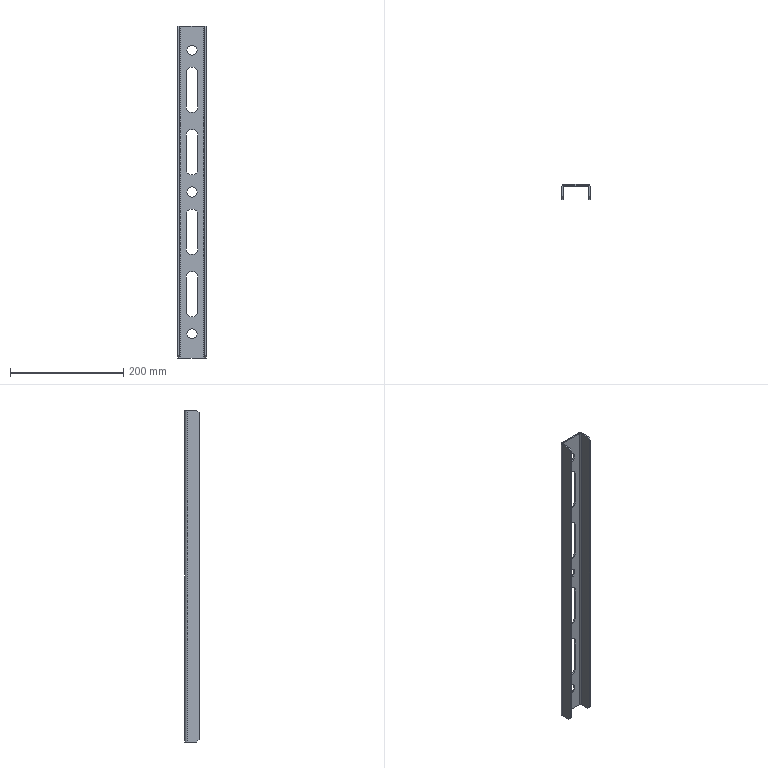Part | SolidWorks | features Chamfer 1, FlatPattern 1, ICE 1, SMBaseFlange 1, SheetMetal 1 | 1 solid | 48 faces | box 50 x 26 x 585.4 mm | volume 111122 mm3 | plane 30 | cylinder 18 | commonest cylinder face diameters 20 x8 18 x6 5 x2 9.6 x2
STEP:
#1=CARTESIAN_POINT('',(-9.,-2.3,-250.));
#2=VERTEX_POINT('',#1);
#3=CARTESIAN_POINT('',(9.,-2.3,-250.));
#4=VERTEX_POINT('',#3);
#5=CARTESIAN_POINT('',(0.,-2.3,-250.));
#6=DIRECTION('',(0.,-1.,0.));
#7=DIRECTION('',(1.,0.,0.));
#8=AXIS2_PLACEMENT_3D('',#5,#6,#7);
#9=CIRCLE('',#8,9.);
#10=EDGE_CURVE('',#2,#4,#9,.T.);
#11=ORIENTED_EDGE('',*,*,#10,.T.);
#12=CARTESIAN_POINT('',(9.,0.,-250.));
#13=VERTEX_POINT('',#12);
#14=CARTESIAN_POINT('',(9.,-26.,-250.));
#15=DIRECTION('',(0.,1.,0.));
#16=VECTOR('',#15,1000.);
#17=LINE('',#14,#16);
#18=EDGE_CURVE('',#4,#13,#17,.T.);
#19=ORIENTED_EDGE('',*,*,#18,.T.);
#20=CARTESIAN_POINT('',(-9.,0.,-250.));
#21=VERTEX_POINT('',#20);
#22=CARTESIAN_POINT('',(0.,0.,-250.));
#23=DIRECTION('',(0.,1.,0.));
#24=DIRECTION('',(1.,0.,0.));
#25=AXIS2_PLACEMENT_3D('',#22,#23,#24);
#26=CIRCLE('',#25,9.);
#27=EDGE_CURVE('',#13,#21,#26,.T.);
#28=ORIENTED_EDGE('',*,*,#27,.T.);
#29=CARTESIAN_POINT('',(-9.,-26.,-250.));
#30=DIRECTION('',(0.,1.,0.));
#31=VECTOR('',#30,1000.);
#32=LINE('',#29,#31);
#33=EDGE_CURVE('',#2,#21,#32,.T.);
#34=ORIENTED_EDGE('',*,*,#33,.F.);
#35=EDGE_LOOP('',(#11,#19,#28,#34));
#36=FACE_OUTER_BOUND('',#35,.T.);
#37=CARTESIAN_POINT('',(0.,-26.,-250.));
#38=DIRECTION('',(0.,1.,0.));
#39=DIRECTION('',(-1.,0.,0.));
#40=AXIS2_PLACEMENT_3D('',#37,#38,#39);
#41=CYLINDRICAL_SURFACE('',#40,9.);
#42=ADVANCED_FACE('',(#36),#41,.F.);
#43=CARTESIAN_POINT('',(-9.,-2.3,250.));
#44=VERTEX_POINT('',#43);
#45=CARTESIAN_POINT('',(9.,-2.3,250.));
#46=VERTEX_POINT('',#45);
#47=CARTESIAN_POINT('',(0.,-2.3,250.));
#48=DIRECTION('',(0.,-1.,0.));
#49=DIRECTION('',(1.,0.,0.));
#50=AXIS2_PLACEMENT_3D('',#47,#48,#49);
#51=CIRCLE('',#50,9.);
#52=EDGE_CURVE('',#44,#46,#51,.T.);
#53=ORIENTED_EDGE('',*,*,#52,.T.);
#54=CARTESIAN_POINT('',(9.,0.,250.));
#55=VERTEX_POINT('',#54);
#56=CARTESIAN_POINT('',(9.,-26.,250.));
#57=DIRECTION('',(0.,1.,0.));
#58=VECTOR('',#57,1000.);
#59=LINE('',#56,#58);
#60=EDGE_CURVE('',#46,#55,#59,.T.);
#61=ORIENTED_EDGE('',*,*,#60,.T.);
#62=CARTESIAN_POINT('',(-9.,0.,250.));
#63=VERTEX_POINT('',#62);
#64=CARTESIAN_POINT('',(0.,0.,250.));
#65=DIRECTION('',(0.,1.,0.));
#66=DIRECTION('',(-1.,0.,0.));
#67=AXIS2_PLACEMENT_3D('',#64,#65,#66);
#68=CIRCLE('',#67,9.);
#69=EDGE_CURVE('',#55,#63,#68,.T.);
#70=ORIENTED_EDGE('',*,*,#69,.T.);
#71=CARTESIAN_POINT('',(-9.,-26.,250.));
#72=DIRECTION('',(0.,1.,0.));
#73=VECTOR('',#72,1000.);
#74=LINE('',#71,#73);
#75=EDGE_CURVE('',#44,#63,#74,.T.);
#76=ORIENTED_EDGE('',*,*,#75,.F.);
#77=EDGE_LOOP('',(#53,#61,#70,#76));
#78=FACE_OUTER_BOUND('',#77,.T.);
#79=CARTESIAN_POINT('',(0.,-26.,250.));
#80=DIRECTION('',(0.,1.,0.));
#81=DIRECTION('',(-1.,0.,0.));
#82=AXIS2_PLACEMENT_3D('',#79,#80,#81);
#83=CYLINDRICAL_SURFACE('',#82,9.);
#84=ADVANCED_FACE('',(#78),#83,.F.);
#85=CARTESIAN_POINT('',(-9.,-2.3,0.));
#86=VERTEX_POINT('',#85);
#87=CARTESIAN_POINT('',(9.,-2.3,0.));
#88=VERTEX_POINT('',#87);
#89=CARTESIAN_POINT('',(0.,-2.3,0.));
#90=DIRECTION('',(0.,-1.,0.));
#91=DIRECTION('',(1.,0.,0.));
#92=AXIS2_PLACEMENT_3D('',#89,#90,#91);
#93=CIRCLE('',#92,9.);
#94=EDGE_CURVE('',#86,#88,#93,.T.);
#95=ORIENTED_EDGE('',*,*,#94,.T.);
#96=CARTESIAN_POINT('',(9.,0.,0.));
#97=VERTEX_POINT('',#96);
#98=CARTESIAN_POINT('',(9.,-26.,0.));
#99=DIRECTION('',(0.,1.,0.));
#100=VECTOR('',#99,1000.);
#101=LINE('',#98,#100);
#102=EDGE_CURVE('',#88,#97,#101,.T.);
#103=ORIENTED_EDGE('',*,*,#102,.T.);
#104=CARTESIAN_POINT('',(-9.,0.,0.));
#105=VERTEX_POINT('',#104);
#106=CARTESIAN_POINT('',(0.,0.,0.));
#107=DIRECTION('',(0.,1.,0.));
#108=DIRECTION('',(-1.,0.,0.));
#109=AXIS2_PLACEMENT_3D('',#106,#107,#108);
#110=CIRCLE('',#109,9.);
#111=EDGE_CURVE('',#97,#105,#110,.T.);
#112=ORIENTED_EDGE('',*,*,#111,.T.);
#113=CARTESIAN_POINT('',(-9.,-26.,0.));
#114=DIRECTION('',(0.,1.,0.));
#115=VECTOR('',#114,1000.);
#116=LINE('',#113,#115);
#117=EDGE_CURVE('',#86,#105,#116,.T.);
#118=ORIENTED_EDGE('',*,*,#117,.F.);
#119=EDGE_LOOP('',(#95,#103,#112,#118));
#120=FACE_OUTER_BOUND('',#119,.T.);
#121=CARTESIAN_POINT('',(0.,-26.,0.));
#122=DIRECTION('',(0.,1.,0.));
#123=DIRECTION('',(-1.,0.,0.));
#124=AXIS2_PLACEMENT_3D('',#121,#122,#123);
#125=CYLINDRICAL_SURFACE('',#124,9.);
#126=ADVANCED_FACE('',(#120),#125,.F.);
#127=CARTESIAN_POINT('',(25.,-4.8,292.7));
#128=VERTEX_POINT('',#127);
#129=CARTESIAN_POINT('',(22.7,-4.8,292.7));
#130=VERTEX_POINT('',#129);
#131=CARTESIAN_POINT('',(25.,-4.8,292.7));
#132=DIRECTION('',(-1.,0.,0.));
#133=VECTOR('',#132,1000.);
#134=LINE('',#131,#133);
#135=EDGE_CURVE('',#128,#130,#134,.T.);
#136=ORIENTED_EDGE('',*,*,#135,.F.);
#137=CARTESIAN_POINT('',(20.2,0.,292.7));
#138=VERTEX_POINT('',#137);
#139=CARTESIAN_POINT('',(20.2,-4.8,292.7));
#140=DIRECTION('',(0.,0.,1.));
#141=DIRECTION('',(-1.,0.,0.));
#142=AXIS2_PLACEMENT_3D('',#139,#140,#141);
#143=CIRCLE('',#142,4.8);
#144=EDGE_CURVE('',#128,#138,#143,.T.);
#145=ORIENTED_EDGE('',*,*,#144,.T.);
#146=CARTESIAN_POINT('',(20.2,-2.3,292.7));
#147=VERTEX_POINT('',#146);
#148=CARTESIAN_POINT('',(20.2,-2.3,292.7));
#149=DIRECTION('',(0.,1.,0.));
#150=VECTOR('',#149,1000.);
#151=LINE('',#148,#150);
#152=EDGE_CURVE('',#147,#138,#151,.T.);
#153=ORIENTED_EDGE('',*,*,#152,.F.);
#154=CARTESIAN_POINT('',(20.2,-4.8,292.7));
#155=DIRECTION('',(0.,0.,1.));
#156=DIRECTION('',(1.,0.,0.));
#157=AXIS2_PLACEMENT_3D('',#154,#155,#156);
#158=CIRCLE('',#157,2.5);
#159=EDGE_CURVE('',#130,#147,#158,.T.);
#160=ORIENTED_EDGE('',*,*,#159,.F.);
#161=EDGE_LOOP('',(#136,#145,#153,#160));
#162=FACE_OUTER_BOUND('',#161,.T.);
#163=CARTESIAN_POINT('',(25.,-4.8,292.7));
#164=DIRECTION('',(0.,0.,1.));
#165=DIRECTION('',(1.,0.,0.));
#166=AXIS2_PLACEMENT_3D('',#163,#164,#165);
#167=PLANE('',#166);
#168=ADVANCED_FACE('',(#162),#167,.T.);
#169=CARTESIAN_POINT('',(22.7,-21.,292.7));
#170=VERTEX_POINT('',#169);
#171=CARTESIAN_POINT('',(22.7,0.,292.7));
#172=DIRECTION('',(0.,1.,0.));
#173=VECTOR('',#172,1000.);
#174=LINE('',#171,#173);
#175=EDGE_CURVE('',#170,#130,#174,.T.);
#176=ORIENTED_EDGE('',*,*,#175,.F.);
#177=CARTESIAN_POINT('',(25.,-21.,292.7));
#178=VERTEX_POINT('',#177);
#179=CARTESIAN_POINT('',(20.2,-21.,292.7));
#180=DIRECTION('',(1.,0.,0.));
#181=VECTOR('',#180,1000.);
#182=LINE('',#179,#181);
#183=EDGE_CURVE('',#170,#178,#182,.T.);
#184=ORIENTED_EDGE('',*,*,#183,.T.);
#185=CARTESIAN_POINT('',(25.,0.,292.7));
#186=DIRECTION('',(0.,1.,0.));
#187=VECTOR('',#186,1000.);
#188=LINE('',#185,#187);
#189=EDGE_CURVE('',#178,#128,#188,.T.);
#190=ORIENTED_EDGE('',*,*,#189,.T.);
#191=ORIENTED_EDGE('',*,*,#135,.T.);
#192=EDGE_LOOP('',(#176,#184,#190,#191));
#193=FACE_OUTER_BOUND('',#192,.T.);
#194=CARTESIAN_POINT('',(20.2,-2.3,292.7));
#195=DIRECTION('',(0.,0.,1.));
#196=DIRECTION('',(1.,0.,0.));
#197=AXIS2_PLACEMENT_3D('',#194,#195,#196);
#198=PLANE('',#197);
#199=ADVANCED_FACE('',(#193),#198,.T.);
#200=CARTESIAN_POINT('',(20.2,0.,-292.7));
#201=VERTEX_POINT('',#200);
#202=CARTESIAN_POINT('',(20.2,-2.3,-292.7));
#203=VERTEX_POINT('',#202);
#204=CARTESIAN_POINT('',(20.2,0.,-292.7));
#205=DIRECTION('',(0.,-1.,0.));
#206=VECTOR('',#205,1000.);
#207=LINE('',#204,#206);
#208=EDGE_CURVE('',#201,#203,#207,.T.);
#209=ORIENTED_EDGE('',*,*,#208,.F.);
#210=CARTESIAN_POINT('',(25.,-4.8,-292.7));
#211=VERTEX_POINT('',#210);
#212=CARTESIAN_POINT('',(20.2,-4.8,-292.7));
#213=DIRECTION('',(0.,0.,1.));
#214=DIRECTION('',(-1.,0.,0.));
#215=AXIS2_PLACEMENT_3D('',#212,#213,#214);
#216=CIRCLE('',#215,4.8);
#217=EDGE_CURVE('',#211,#201,#216,.T.);
#218=ORIENTED_EDGE('',*,*,#217,.F.);
#219=CARTESIAN_POINT('',(22.7,-4.8,-292.7));
#220=VERTEX_POINT('',#219);
#221=CARTESIAN_POINT('',(22.7,-4.8,-292.7));
#222=DIRECTION('',(1.,0.,0.));
#223=VECTOR('',#222,1000.);
#224=LINE('',#221,#223);
#225=EDGE_CURVE('',#220,#211,#224,.T.);
#226=ORIENTED_EDGE('',*,*,#225,.F.);
#227=CARTESIAN_POINT('',(20.2,-4.8,-292.7));
#228=DIRECTION('',(0.,0.,1.));
#229=DIRECTION('',(1.,0.,0.));
#230=AXIS2_PLACEMENT_3D('',#227,#228,#229);
#231=CIRCLE('',#230,2.5);
#232=EDGE_CURVE('',#220,#203,#231,.T.);
#233=ORIENTED_EDGE('',*,*,#232,.T.);
#234=EDGE_LOOP('',(#209,#218,#226,#233));
#235=FACE_OUTER_BOUND('',#234,.T.);
#236=CARTESIAN_POINT('',(20.2,0.,-292.7));
#237=DIRECTION('',(0.,0.,-1.));
#238=DIRECTION('',(-1.,0.,0.));
#239=AXIS2_PLACEMENT_3D('',#236,#237,#238);
#240=PLANE('',#239);
#241=ADVANCED_FACE('',(#235),#240,.T.);
#242=CARTESIAN_POINT('',(-20.2,0.,-292.7));
#243=VERTEX_POINT('',#242);
#244=CARTESIAN_POINT('',(-25.,0.,-292.7));
#245=DIRECTION('',(-1.,0.,0.));
#246=VECTOR('',#245,1000.);
#247=LINE('',#244,#246);
#248=EDGE_CURVE('',#201,#243,#247,.T.);
#249=ORIENTED_EDGE('',*,*,#248,.F.);
#250=ORIENTED_EDGE('',*,*,#208,.T.);
#251=CARTESIAN_POINT('',(-20.2,-2.3,-292.7));
#252=VERTEX_POINT('',#251);
#253=CARTESIAN_POINT('',(-25.,-2.3,-292.7));
#254=DIRECTION('',(-1.,0.,0.));
#255=VECTOR('',#254,1000.);
#256=LINE('',#253,#255);
#257=EDGE_CURVE('',#203,#252,#256,.T.);
#258=ORIENTED_EDGE('',*,*,#257,.T.);
#259=CARTESIAN_POINT('',(-20.2,-2.3,-292.7));
#260=DIRECTION('',(0.,1.,0.));
#261=VECTOR('',#260,1000.);
#262=LINE('',#259,#261);
#263=EDGE_CURVE('',#252,#243,#262,.T.);
#264=ORIENTED_EDGE('',*,*,#263,.T.);
#265=EDGE_LOOP('',(#249,#250,#258,#264));
#266=FACE_OUTER_BOUND('',#265,.T.);
#267=CARTESIAN_POINT('',(22.7,-4.8,-292.7));
#268=DIRECTION('',(0.,0.,-1.));
#269=DIRECTION('',(-1.,0.,0.));
#270=AXIS2_PLACEMENT_3D('',#267,#268,#269);
#271=PLANE('',#270);
#272=ADVANCED_FACE('',(#266),#271,.T.);
#273=CARTESIAN_POINT('',(-20.2,0.,292.7));
#274=VERTEX_POINT('',#273);
#275=CARTESIAN_POINT('',(-20.2,-2.3,292.7));
#276=VERTEX_POINT('',#275);
#277=CARTESIAN_POINT('',(-20.2,0.,292.7));
#278=DIRECTION('',(0.,-1.,0.));
#279=VECTOR('',#278,1000.);
#280=LINE('',#277,#279);
#281=EDGE_CURVE('',#274,#276,#280,.T.);
#282=ORIENTED_EDGE('',*,*,#281,.F.);
#283=CARTESIAN_POINT('',(-25.,-4.8,292.7));
#284=VERTEX_POINT('',#283);
#285=CARTESIAN_POINT('',(-20.2,-4.8,292.7));
#286=DIRECTION('',(0.,0.,1.));
#287=DIRECTION('',(-1.,0.,0.));
#288=AXIS2_PLACEMENT_3D('',#285,#286,#287);
#289=CIRCLE('',#288,4.8);
#290=EDGE_CURVE('',#274,#284,#289,.T.);
#291=ORIENTED_EDGE('',*,*,#290,.T.);
#292=CARTESIAN_POINT('',(-22.7,-4.8,292.7));
#293=VERTEX_POINT('',#292);
#294=CARTESIAN_POINT('',(-22.7,-4.8,292.7));
#295=DIRECTION('',(-1.,0.,0.));
#296=VECTOR('',#295,1000.);
#297=LINE('',#294,#296);
#298=EDGE_CURVE('',#293,#284,#297,.T.);
#299=ORIENTED_EDGE('',*,*,#298,.F.);
#300=CARTESIAN_POINT('',(-20.2,-4.8,292.7));
#301=DIRECTION('',(0.,0.,1.));
#302=DIRECTION('',(1.,0.,0.));
#303=AXIS2_PLACEMENT_3D('',#300,#301,#302);
#304=CIRCLE('',#303,2.5);
#305=EDGE_CURVE('',#276,#293,#304,.T.);
#306=ORIENTED_EDGE('',*,*,#305,.F.);
#307=EDGE_LOOP('',(#282,#291,#299,#306));
#308=FACE_OUTER_BOUND('',#307,.T.);
#309=CARTESIAN_POINT('',(-20.2,0.,292.7));
#310=DIRECTION('',(0.,0.,1.));
#311=DIRECTION('',(1.,0.,0.));
#312=AXIS2_PLACEMENT_3D('',#309,#310,#311);
#313=PLANE('',#312);
#314=ADVANCED_FACE('',(#308),#313,.T.);
#315=CARTESIAN_POINT('',(-25.,0.,292.7));
#316=DIRECTION('',(-1.,0.,0.));
#317=VECTOR('',#316,1000.);
#318=LINE('',#315,#317);
#319=EDGE_CURVE('',#138,#274,#318,.T.);
#320=ORIENTED_EDGE('',*,*,#319,.T.);
#321=ORIENTED_EDGE('',*,*,#281,.T.);
#322=CARTESIAN_POINT('',(-25.,-2.3,292.7));
#323=DIRECTION('',(-1.,0.,0.));
#324=VECTOR('',#323,1000.);
#325=LINE('',#322,#324);
#326=EDGE_CURVE('',#147,#276,#325,.T.);
#327=ORIENTED_EDGE('',*,*,#326,.F.);
#328=ORIENTED_EDGE('',*,*,#152,.T.);
#329=EDGE_LOOP('',(#320,#321,#327,#328));
#330=FACE_OUTER_BOUND('',#329,.T.);
#331=CARTESIAN_POINT('',(-22.7,-4.8,292.7));
#332=DIRECTION('',(0.,0.,1.));
#333=DIRECTION('',(1.,0.,0.));
#334=AXIS2_PLACEMENT_3D('',#331,#332,#333);
#335=PLANE('',#334);
#336=ADVANCED_FACE('',(#330),#335,.T.);
#337=CARTESIAN_POINT('',(-25.,-4.8,-292.7));
#338=VERTEX_POINT('',#337);
#339=CARTESIAN_POINT('',(-22.7,-4.8,-292.7));
#340=VERTEX_POINT('',#339);
#341=CARTESIAN_POINT('',(-25.,-4.8,-292.7));
#342=DIRECTION('',(1.,0.,0.));
#343=VECTOR('',#342,1000.);
#344=LINE('',#341,#343);
#345=EDGE_CURVE('',#338,#340,#344,.T.);
#346=ORIENTED_EDGE('',*,*,#345,.F.);
#347=CARTESIAN_POINT('',(-20.2,-4.8,-292.7));
#348=DIRECTION('',(0.,0.,1.));
#349=DIRECTION('',(-1.,0.,0.));
#350=AXIS2_PLACEMENT_3D('',#347,#348,#349);
#351=CIRCLE('',#350,4.8);
#352=EDGE_CURVE('',#243,#338,#351,.T.);
#353=ORIENTED_EDGE('',*,*,#352,.F.);
#354=ORIENTED_EDGE('',*,*,#263,.F.);
#355=CARTESIAN_POINT('',(-20.2,-4.8,-292.7));
#356=DIRECTION('',(0.,0.,1.));
#357=DIRECTION('',(1.,0.,0.));
#358=AXIS2_PLACEMENT_3D('',#355,#356,#357);
#359=CIRCLE('',#358,2.5);
#360=EDGE_CURVE('',#252,#340,#359,.T.);
#361=ORIENTED_EDGE('',*,*,#360,.T.);
#362=EDGE_LOOP('',(#346,#353,#354,#361));
#363=FACE_OUTER_BOUND('',#362,.T.);
#364=CARTESIAN_POINT('',(-25.,-4.8,-292.7));
#365=DIRECTION('',(0.,0.,-1.));
#366=DIRECTION('',(-1.,0.,0.));
#367=AXIS2_PLACEMENT_3D('',#364,#365,#366);
#368=PLANE('',#367);
#369=ADVANCED_FACE('',(#363),#368,.T.);
#370=CARTESIAN_POINT('',(-22.7,-21.,-292.7));
#371=VERTEX_POINT('',#370);
#372=CARTESIAN_POINT('',(-22.7,0.,-292.7));
#373=DIRECTION('',(0.,-1.,0.));
#374=VECTOR('',#373,1000.);
#375=LINE('',#372,#374);
#376=EDGE_CURVE('',#340,#371,#375,.T.);
#377=ORIENTED_EDGE('',*,*,#376,.T.);
#378=CARTESIAN_POINT('',(-25.,-21.,-292.7));
#379=VERTEX_POINT('',#378);
#380=CARTESIAN_POINT('',(-20.2,-21.,-292.7));
#381=DIRECTION('',(-1.,0.,0.));
#382=VECTOR('',#381,1000.);
#383=LINE('',#380,#382);
#384=EDGE_CURVE('',#371,#379,#383,.T.);
#385=ORIENTED_EDGE('',*,*,#384,.T.);
#386=CARTESIAN_POINT('',(-25.,0.,-292.7));
#387=DIRECTION('',(0.,-1.,0.));
#388=VECTOR('',#387,1000.);
#389=LINE('',#386,#388);
#390=EDGE_CURVE('',#338,#379,#389,.T.);
#391=ORIENTED_EDGE('',*,*,#390,.F.);
#392=ORIENTED_EDGE('',*,*,#345,.T.);
#393=EDGE_LOOP('',(#377,#385,#391,#392));
#394=FACE_OUTER_BOUND('',#393,.T.);
#395=CARTESIAN_POINT('',(-20.2,-2.3,-292.7));
#396=DIRECTION('',(0.,0.,-1.));
#397=DIRECTION('',(-1.,0.,0.));
#398=AXIS2_PLACEMENT_3D('',#395,#396,#397);
#399=PLANE('',#398);
#400=ADVANCED_FACE('',(#394),#399,.T.);
#401=ORIENTED_EDGE('',*,*,#390,.T.);
#402=CARTESIAN_POINT('',(-25.,-26.,-287.7));
#403=VERTEX_POINT('',#402);
#404=CARTESIAN_POINT('',(-25.,-21.,-292.7));
#405=DIRECTION('',(0.,-0.7071,0.7071));
#406=VECTOR('',#405,1000.);
#407=LINE('',#404,#406);
#408=EDGE_CURVE('',#379,#403,#407,.T.);
#409=ORIENTED_EDGE('',*,*,#408,.T.);
#410=CARTESIAN_POINT('',(-25.,-26.,287.7));
#411=VERTEX_POINT('',#410);
#412=CARTESIAN_POINT('',(-25.,-26.,292.7));
#413=DIRECTION('',(0.,0.,-1.));
#414=VECTOR('',#413,1000.);
#415=LINE('',#412,#414);
#416=EDGE_CURVE('',#411,#403,#415,.T.);
#417=ORIENTED_EDGE('',*,*,#416,.F.);
#418=CARTESIAN_POINT('',(-25.,-21.,292.7));
#419=VERTEX_POINT('',#418);
#420=CARTESIAN_POINT('',(-25.,-26.,287.7));
#421=DIRECTION('',(0.,0.7071,0.7071));
#422=VECTOR('',#421,1000.);
#423=LINE('',#420,#422);
#424=EDGE_CURVE('',#411,#419,#423,.T.);
#425=ORIENTED_EDGE('',*,*,#424,.T.);
#426=CARTESIAN_POINT('',(-25.,0.,292.7));
#427=DIRECTION('',(0.,-1.,0.));
#428=VECTOR('',#427,1000.);
#429=LINE('',#426,#428);
#430=EDGE_CURVE('',#284,#419,#429,.T.);
#431=ORIENTED_EDGE('',*,*,#430,.F.);
#432=CARTESIAN_POINT('',(-25.,-4.8,292.7));
#433=DIRECTION('',(0.,0.,-1.));
#434=VECTOR('',#433,1000.);
#435=LINE('',#432,#434);
#436=EDGE_CURVE('',#284,#338,#435,.T.);
#437=ORIENTED_EDGE('',*,*,#436,.T.);
#438=EDGE_LOOP('',(#401,#409,#417,#425,#431,#437));
#439=FACE_OUTER_BOUND('',#438,.T.);
#440=CARTESIAN_POINT('',(-25.,0.,292.7));
#441=DIRECTION('',(1.,0.,0.));
#442=DIRECTION('',(0.,0.,-1.));
#443=AXIS2_PLACEMENT_3D('',#440,#441,#442);
#444=PLANE('',#443);
#445=ADVANCED_FACE('',(#439),#444,.F.);
#446=ORIENTED_EDGE('',*,*,#416,.T.);
#447=CARTESIAN_POINT('',(-22.7,-26.,-287.7));
#448=VERTEX_POINT('',#447);
#449=CARTESIAN_POINT('',(-22.7,-26.,-287.7));
#450=DIRECTION('',(1.,0.,0.));
#451=VECTOR('',#450,1000.);
#452=LINE('',#449,#451);
#453=EDGE_CURVE('',#403,#448,#452,.T.);
#454=ORIENTED_EDGE('',*,*,#453,.T.);
#455=CARTESIAN_POINT('',(-22.7,-26.,287.7));
#456=VERTEX_POINT('',#455);
#457=CARTESIAN_POINT('',(-22.7,-26.,292.7));
#458=DIRECTION('',(0.,0.,-1.));
#459=VECTOR('',#458,1000.);
#460=LINE('',#457,#459);
#461=EDGE_CURVE('',#456,#448,#460,.T.);
#462=ORIENTED_EDGE('',*,*,#461,.F.);
#463=CARTESIAN_POINT('',(-22.7,-26.,287.7));
#464=DIRECTION('',(-1.,0.,0.));
#465=VECTOR('',#464,1000.);
#466=LINE('',#463,#465);
#467=EDGE_CURVE('',#456,#411,#466,.T.);
#468=ORIENTED_EDGE('',*,*,#467,.T.);
#469=EDGE_LOOP('',(#446,#454,#462,#468));
#470=FACE_OUTER_BOUND('',#469,.T.);
#471=CARTESIAN_POINT('',(-22.7,-26.,292.7));
#472=DIRECTION('',(0.,-1.,0.));
#473=DIRECTION('',(0.,0.,-1.));
#474=AXIS2_PLACEMENT_3D('',#471,#472,#473);
#475=PLANE('',#474);
#476=ADVANCED_FACE('',(#470),#475,.T.);
#477=ORIENTED_EDGE('',*,*,#461,.T.);
#478=CARTESIAN_POINT('',(-22.7,-303.2,-10.5));
#479=DIRECTION('',(0.,0.7071,-0.7071));
#480=VECTOR('',#479,1000.);
#481=LINE('',#478,#480);
#482=EDGE_CURVE('',#448,#371,#481,.T.);
#483=ORIENTED_EDGE('',*,*,#482,.T.);
#484=ORIENTED_EDGE('',*,*,#376,.F.);
#485=CARTESIAN_POINT('',(-22.7,-4.8,292.7));
#486=DIRECTION('',(0.,0.,-1.));
#487=VECTOR('',#486,1000.);
#488=LINE('',#485,#487);
#489=EDGE_CURVE('',#293,#340,#488,.T.);
#490=ORIENTED_EDGE('',*,*,#489,.F.);
#491=CARTESIAN_POINT('',(-22.7,-21.,292.7));
#492=VERTEX_POINT('',#491);
#493=CARTESIAN_POINT('',(-22.7,0.,292.7));
#494=DIRECTION('',(0.,-1.,0.));
#495=VECTOR('',#494,1000.);
#496=LINE('',#493,#495);
#497=EDGE_CURVE('',#293,#492,#496,.T.);
#498=ORIENTED_EDGE('',*,*,#497,.T.);
#499=CARTESIAN_POINT('',(-22.7,-10.5,303.2));
#500=DIRECTION('',(0.,-0.7071,-0.7071));
#501=VECTOR('',#500,1000.);
#502=LINE('',#499,#501);
#503=EDGE_CURVE('',#492,#456,#502,.T.);
#504=ORIENTED_EDGE('',*,*,#503,.T.);
#505=EDGE_LOOP('',(#477,#483,#484,#490,#498,#504));
#506=FACE_OUTER_BOUND('',#505,.T.);
#507=CARTESIAN_POINT('',(-22.7,0.,292.7));
#508=DIRECTION('',(1.,0.,0.));
#509=DIRECTION('',(0.,0.,-1.));
#510=AXIS2_PLACEMENT_3D('',#507,#508,#509);
#511=PLANE('',#510);
#512=ADVANCED_FACE('',(#506),#511,.T.);
#513=ORIENTED_EDGE('',*,*,#360,.F.);
#514=CARTESIAN_POINT('',(-20.2,-2.3,292.7));
#515=DIRECTION('',(0.,0.,-1.));
#516=VECTOR('',#515,1000.);
#517=LINE('',#514,#516);
#518=EDGE_CURVE('',#276,#252,#517,.T.);
#519=ORIENTED_EDGE('',*,*,#518,.F.);
#520=ORIENTED_EDGE('',*,*,#305,.T.);
#521=ORIENTED_EDGE('',*,*,#489,.T.);
#522=EDGE_LOOP('',(#513,#519,#520,#521));
#523=FACE_OUTER_BOUND('',#522,.T.);
#524=CARTESIAN_POINT('',(-20.2,-4.8,292.7));
#525=DIRECTION('',(0.,0.,-1.));
#526=DIRECTION('',(-1.,0.,0.));
#527=AXIS2_PLACEMENT_3D('',#524,#525,#526);
#528=CYLINDRICAL_SURFACE('',#527,2.5);
#529=ADVANCED_FACE('',(#523),#528,.F.);
#530=ORIENTED_EDGE('',*,*,#10,.F.);
#531=CARTESIAN_POINT('',(0.,-2.3,-250.));
#532=DIRECTION('',(0.,-1.,0.));
#533=DIRECTION('',(1.,0.,0.));
#534=AXIS2_PLACEMENT_3D('',#531,#532,#533);
#535=CIRCLE('',#534,9.);
#536=EDGE_CURVE('',#4,#2,#535,.T.);
#537=ORIENTED_EDGE('',*,*,#536,.F.);
#538=EDGE_LOOP('',(#530,#537));
#539=FACE_BOUND('',#538,.T.);
#540=CARTESIAN_POINT('',(10.,-2.3,-150.));
#541=VERTEX_POINT('',#540);
#542=CARTESIAN_POINT('',(-10.,-2.3,-150.));
#543=VERTEX_POINT('',#542);
#544=CARTESIAN_POINT('',(0.,-2.3,-150.));
#545=DIRECTION('',(0.,-1.,0.));
#546=DIRECTION('',(1.,0.,0.));
#547=AXIS2_PLACEMENT_3D('',#544,#545,#546);
#548=CIRCLE('',#547,10.);
#549=EDGE_CURVE('',#541,#543,#548,.T.);
#550=ORIENTED_EDGE('',*,*,#549,.F.);
#551=CARTESIAN_POINT('',(10.,-2.3,-210.));
#552=VERTEX_POINT('',#551);
#553=CARTESIAN_POINT('',(10.,-2.3,292.7));
#554=DIRECTION('',(0.,0.,1.));
#555=VECTOR('',#554,1000.);
#556=LINE('',#553,#555);
#557=EDGE_CURVE('',#552,#541,#556,.T.);
#558=ORIENTED_EDGE('',*,*,#557,.F.);
#559=CARTESIAN_POINT('',(-10.,-2.3,-210.));
#560=VERTEX_POINT('',#559);
#561=CARTESIAN_POINT('',(0.,-2.3,-210.));
#562=DIRECTION('',(0.,-1.,0.));
#563=DIRECTION('',(1.,0.,0.));
#564=AXIS2_PLACEMENT_3D('',#561,#562,#563);
#565=CIRCLE('',#564,10.);
#566=EDGE_CURVE('',#560,#552,#565,.T.);
#567=ORIENTED_EDGE('',*,*,#566,.F.);
#568=CARTESIAN_POINT('',(-10.,-2.3,292.7));
#569=DIRECTION('',(0.,0.,-1.));
#570=VECTOR('',#569,1000.);
#571=LINE('',#568,#570);
#572=EDGE_CURVE('',#543,#560,#571,.T.);
#573=ORIENTED_EDGE('',*,*,#572,.F.);
#574=EDGE_LOOP('',(#550,#558,#567,#573));
#575=FACE_BOUND('',#574,.T.);
#576=CARTESIAN_POINT('',(-10.,-2.3,40.));
#577=VERTEX_POINT('',#576);
#578=CARTESIAN_POINT('',(10.,-2.3,40.));
#579=VERTEX_POINT('',#578);
#580=CARTESIAN_POINT('',(0.,-2.3,40.));
#581=DIRECTION('',(0.,-1.,0.));
#582=DIRECTION('',(1.,0.,0.));
#583=AXIS2_PLACEMENT_3D('',#580,#581,#582);
#584=CIRCLE('',#583,10.);
#585=EDGE_CURVE('',#577,#579,#584,.T.);
#586=ORIENTED_EDGE('',*,*,#585,.F.);
#587=CARTESIAN_POINT('',(-10.,-2.3,100.));
#588=VERTEX_POINT('',#587);
#589=CARTESIAN_POINT('',(-10.,-2.3,292.7));
#590=DIRECTION('',(0.,0.,-1.));
#591=VECTOR('',#590,1000.);
#592=LINE('',#589,#591);
#593=EDGE_CURVE('',#588,#577,#592,.T.);
#594=ORIENTED_EDGE('',*,*,#593,.F.);
#595=CARTESIAN_POINT('',(10.,-2.3,100.));
#596=VERTEX_POINT('',#595);
#597=CARTESIAN_POINT('',(0.,-2.3,100.));
#598=DIRECTION('',(0.,-1.,0.));
#599=DIRECTION('',(1.,0.,0.));
#600=AXIS2_PLACEMENT_3D('',#597,#598,#599);
#601=CIRCLE('',#600,10.);
#602=EDGE_CURVE('',#596,#588,#601,.T.);
#603=ORIENTED_EDGE('',*,*,#602,.F.);
#604=CARTESIAN_POINT('',(10.,-2.3,292.7));
#605=DIRECTION('',(0.,0.,1.));
#606=VECTOR('',#605,1000.);
#607=LINE('',#604,#606);
#608=EDGE_CURVE('',#579,#596,#607,.T.);
#609=ORIENTED_EDGE('',*,*,#608,.F.);
#610=EDGE_LOOP('',(#586,#594,#603,#609));
#611=FACE_BOUND('',#610,.T.);
#612=ORIENTED_EDGE('',*,*,#52,.F.);
#613=CARTESIAN_POINT('',(0.,-2.3,250.));
#614=DIRECTION('',(0.,-1.,0.));
#615=DIRECTION('',(1.,0.,0.));
#616=AXIS2_PLACEMENT_3D('',#613,#614,#615);
#617=CIRCLE('',#616,9.);
#618=EDGE_CURVE('',#46,#44,#617,.T.);
#619=ORIENTED_EDGE('',*,*,#618,.F.);
#620=EDGE_LOOP('',(#612,#619));
#621=FACE_BOUND('',#620,.T.);
#622=CARTESIAN_POINT('',(-10.,-2.3,150.));
#623=VERTEX_POINT('',#622);
#624=CARTESIAN_POINT('',(10.,-2.3,150.));
#625=VERTEX_POINT('',#624);
#626=CARTESIAN_POINT('',(0.,-2.3,150.));
#627=DIRECTION('',(0.,-1.,0.));
#628=DIRECTION('',(1.,0.,0.));
#629=AXIS2_PLACEMENT_3D('',#626,#627,#628);
#630=CIRCLE('',#629,10.);
#631=EDGE_CURVE('',#623,#625,#630,.T.);
#632=ORIENTED_EDGE('',*,*,#631,.F.);
#633=CARTESIAN_POINT('',(-10.,-2.3,210.));
#634=VERTEX_POINT('',#633);
#635=CARTESIAN_POINT('',(-10.,-2.3,292.7));
#636=DIRECTION('',(0.,0.,-1.));
#637=VECTOR('',#636,1000.);
#638=LINE('',#635,#637);
#639=EDGE_CURVE('',#634,#623,#638,.T.);
#640=ORIENTED_EDGE('',*,*,#639,.F.);
#641=CARTESIAN_POINT('',(10.,-2.3,210.));
#642=VERTEX_POINT('',#641);
#643=CARTESIAN_POINT('',(0.,-2.3,210.));
#644=DIRECTION('',(0.,-1.,0.));
#645=DIRECTION('',(1.,0.,0.));
#646=AXIS2_PLACEMENT_3D('',#643,#644,#645);
#647=CIRCLE('',#646,10.);
#648=EDGE_CURVE('',#642,#634,#647,.T.);
#649=ORIENTED_EDGE('',*,*,#648,.F.);
#650=CARTESIAN_POINT('',(10.,-2.3,292.7));
#651=DIRECTION('',(0.,0.,1.));
#652=VECTOR('',#651,1000.);
#653=LINE('',#650,#652);
#654=EDGE_CURVE('',#625,#642,#653,.T.);
#655=ORIENTED_EDGE('',*,*,#654,.F.);
#656=EDGE_LOOP('',(#632,#640,#649,#655));
#657=FACE_BOUND('',#656,.T.);
#658=CARTESIAN_POINT('',(10.,-2.3,-40.));
#659=VERTEX_POINT('',#658);
#660=CARTESIAN_POINT('',(-10.,-2.3,-40.));
#661=VERTEX_POINT('',#660);
#662=CARTESIAN_POINT('',(0.,-2.3,-40.));
#663=DIRECTION('',(0.,-1.,0.));
#664=DIRECTION('',(1.,0.,0.));
#665=AXIS2_PLACEMENT_3D('',#662,#663,#664);
#666=CIRCLE('',#665,10.);
#667=EDGE_CURVE('',#659,#661,#666,.T.);
#668=ORIENTED_EDGE('',*,*,#667,.F.);
#669=CARTESIAN_POINT('',(10.,-2.3,-100.));
#670=VERTEX_POINT('',#669);
#671=CARTESIAN_POINT('',(10.,-2.3,292.7));
#672=DIRECTION('',(0.,0.,1.));
#673=VECTOR('',#672,1000.);
#674=LINE('',#671,#673);
#675=EDGE_CURVE('',#670,#659,#674,.T.);
#676=ORIENTED_EDGE('',*,*,#675,.F.);
#677=CARTESIAN_POINT('',(-10.,-2.3,-100.));
#678=VERTEX_POINT('',#677);
#679=CARTESIAN_POINT('',(0.,-2.3,-100.));
#680=DIRECTION('',(0.,-1.,0.));
#681=DIRECTION('',(1.,0.,0.));
#682=AXIS2_PLACEMENT_3D('',#679,#680,#681);
#683=CIRCLE('',#682,10.);
#684=EDGE_CURVE('',#678,#670,#683,.T.);
#685=ORIENTED_EDGE('',*,*,#684,.F.);
#686=CARTESIAN_POINT('',(-10.,-2.3,292.7));
#687=DIRECTION('',(0.,0.,-1.));
#688=VECTOR('',#687,1000.);
#689=LINE('',#686,#688);
#690=EDGE_CURVE('',#661,#678,#689,.T.);
#691=ORIENTED_EDGE('',*,*,#690,.F.);
#692=EDGE_LOOP('',(#668,#676,#685,#691));
#693=FACE_BOUND('',#692,.T.);
#694=ORIENTED_EDGE('',*,*,#94,.F.);
#695=CARTESIAN_POINT('',(0.,-2.3,0.));
#696=DIRECTION('',(0.,-1.,0.));
#697=DIRECTION('',(1.,0.,0.));
#698=AXIS2_PLACEMENT_3D('',#695,#696,#697);
#699=CIRCLE('',#698,9.);
#700=EDGE_CURVE('',#88,#86,#699,.T.);
#701=ORIENTED_EDGE('',*,*,#700,.F.);
#702=EDGE_LOOP('',(#694,#701));
#703=FACE_BOUND('',#702,.T.);
#704=ORIENTED_EDGE('',*,*,#257,.F.);
#705=CARTESIAN_POINT('',(20.2,-2.3,292.7));
#706=DIRECTION('',(0.,0.,-1.));
#707=VECTOR('',#706,1000.);
#708=LINE('',#705,#707);
#709=EDGE_CURVE('',#147,#203,#708,.T.);
#710=ORIENTED_EDGE('',*,*,#709,.F.);
#711=ORIENTED_EDGE('',*,*,#326,.T.);
#712=ORIENTED_EDGE('',*,*,#518,.T.);
#713=EDGE_LOOP('',(#704,#710,#711,#712));
#714=FACE_OUTER_BOUND('',#713,.T.);
#715=CARTESIAN_POINT('',(-25.,-2.3,292.7));
#716=DIRECTION('',(0.,-1.,0.));
#717=DIRECTION('',(1.,0.,0.));
#718=AXIS2_PLACEMENT_3D('',#715,#716,#717);
#719=PLANE('',#718);
#720=ADVANCED_FACE('',(#539,#575,#611,#621,#657,#693,#703,#714),#719,.T.);
#721=ORIENTED_EDGE('',*,*,#232,.F.);
#722=CARTESIAN_POINT('',(22.7,-4.8,292.7));
#723=DIRECTION('',(0.,0.,-1.));
#724=VECTOR('',#723,1000.);
#725=LINE('',#722,#724);
#726=EDGE_CURVE('',#130,#220,#725,.T.);
#727=ORIENTED_EDGE('',*,*,#726,.F.);
#728=ORIENTED_EDGE('',*,*,#159,.T.);
#729=ORIENTED_EDGE('',*,*,#709,.T.);
#730=EDGE_LOOP('',(#721,#727,#728,#729));
#731=FACE_OUTER_BOUND('',#730,.T.);
#732=CARTESIAN_POINT('',(20.2,-4.8,292.7));
#733=DIRECTION('',(0.,0.,-1.));
#734=DIRECTION('',(-1.,0.,0.));
#735=AXIS2_PLACEMENT_3D('',#732,#733,#734);
#736=CYLINDRICAL_SURFACE('',#735,2.5);
#737=ADVANCED_FACE('',(#731),#736,.F.);
#738=CARTESIAN_POINT('',(22.7,-21.,-292.7));
#739=VERTEX_POINT('',#738);
#740=CARTESIAN_POINT('',(22.7,0.,-292.7));
#741=DIRECTION('',(0.,1.,0.));
#742=VECTOR('',#741,1000.);
#743=LINE('',#740,#742);
#744=EDGE_CURVE('',#739,#220,#743,.T.);
#745=ORIENTED_EDGE('',*,*,#744,.F.);
#746=CARTESIAN_POINT('',(22.7,-26.,-287.7));
#747=VERTEX_POINT('',#746);
#748=CARTESIAN_POINT('',(22.7,-303.2,-10.5));
#749=DIRECTION('',(0.,-0.7071,0.7071));
#750=VECTOR('',#749,1000.);
#751=LINE('',#748,#750);
#752=EDGE_CURVE('',#739,#747,#751,.T.);
#753=ORIENTED_EDGE('',*,*,#752,.T.);
#754=CARTESIAN_POINT('',(22.7,-26.,287.7));
#755=VERTEX_POINT('',#754);
#756=CARTESIAN_POINT('',(22.7,-26.,292.7));
#757=DIRECTION('',(0.,0.,-1.));
#758=VECTOR('',#757,1000.);
#759=LINE('',#756,#758);
#760=EDGE_CURVE('',#755,#747,#759,.T.);
#761=ORIENTED_EDGE('',*,*,#760,.F.);
#762=CARTESIAN_POINT('',(22.7,-10.5,303.2));
#763=DIRECTION('',(0.,0.7071,0.7071));
#764=VECTOR('',#763,1000.);
#765=LINE('',#762,#764);
#766=EDGE_CURVE('',#755,#170,#765,.T.);
#767=ORIENTED_EDGE('',*,*,#766,.T.);
#768=ORIENTED_EDGE('',*,*,#175,.T.);
#769=ORIENTED_EDGE('',*,*,#726,.T.);
#770=EDGE_LOOP('',(#745,#753,#761,#767,#768,#769));
#771=FACE_OUTER_BOUND('',#770,.T.);
#772=CARTESIAN_POINT('',(22.7,0.,292.7));
#773=DIRECTION('',(-1.,0.,0.));
#774=DIRECTION('',(0.,-1.,0.));
#775=AXIS2_PLACEMENT_3D('',#772,#773,#774);
#776=PLANE('',#775);
#777=ADVANCED_FACE('',(#771),#776,.T.);
#778=ORIENTED_EDGE('',*,*,#760,.T.);
#779=CARTESIAN_POINT('',(25.,-26.,-287.7));
#780=VERTEX_POINT('',#779);
#781=CARTESIAN_POINT('',(25.,-26.,-287.7));
#782=DIRECTION('',(1.,0.,0.));
#783=VECTOR('',#782,1000.);
#784=LINE('',#781,#783);
#785=EDGE_CURVE('',#747,#780,#784,.T.);
#786=ORIENTED_EDGE('',*,*,#785,.T.);
#787=CARTESIAN_POINT('',(25.,-26.,287.7));
#788=VERTEX_POINT('',#787);
#789=CARTESIAN_POINT('',(25.,-26.,292.7));
#790=DIRECTION('',(0.,0.,-1.));
#791=VECTOR('',#790,1000.);
#792=LINE('',#789,#791);
#793=EDGE_CURVE('',#788,#780,#792,.T.);
#794=ORIENTED_EDGE('',*,*,#793,.F.);
#795=CARTESIAN_POINT('',(25.,-26.,287.7));
#796=DIRECTION('',(-1.,0.,0.));
#797=VECTOR('',#796,1000.);
#798=LINE('',#795,#797);
#799=EDGE_CURVE('',#788,#755,#798,.T.);
#800=ORIENTED_EDGE('',*,*,#799,.T.);
#801=EDGE_LOOP('',(#778,#786,#794,#800));
#802=FACE_OUTER_BOUND('',#801,.T.);
#803=CARTESIAN_POINT('',(25.,-26.,292.7));
#804=DIRECTION('',(0.,-1.,0.));
#805=DIRECTION('',(0.,0.,-1.));
#806=AXIS2_PLACEMENT_3D('',#803,#804,#805);
#807=PLANE('',#806);
#808=ADVANCED_FACE('',(#802),#807,.T.);
#809=ORIENTED_EDGE('',*,*,#793,.T.);
#810=CARTESIAN_POINT('',(25.,-21.,-292.7));
#811=VERTEX_POINT('',#810);
#812=CARTESIAN_POINT('',(25.,-21.,-292.7));
#813=DIRECTION('',(0.,0.7071,-0.7071));
#814=VECTOR('',#813,1000.);
#815=LINE('',#812,#814);
#816=EDGE_CURVE('',#780,#811,#815,.T.);
#817=ORIENTED_EDGE('',*,*,#816,.T.);
#818=CARTESIAN_POINT('',(25.,0.,-292.7));
#819=DIRECTION('',(0.,1.,0.));
#820=VECTOR('',#819,1000.);
#821=LINE('',#818,#820);
#822=EDGE_CURVE('',#811,#211,#821,.T.);
#823=ORIENTED_EDGE('',*,*,#822,.T.);
#824=CARTESIAN_POINT('',(25.,-4.8,292.7));
#825=DIRECTION('',(0.,0.,-1.));
#826=VECTOR('',#825,1000.);
#827=LINE('',#824,#826);
#828=EDGE_CURVE('',#128,#211,#827,.T.);
#829=ORIENTED_EDGE('',*,*,#828,.F.);
#830=ORIENTED_EDGE('',*,*,#189,.F.);
#831=CARTESIAN_POINT('',(25.,-26.,287.7));
#832=DIRECTION('',(0.,-0.7071,-0.7071));
#833=VECTOR('',#832,1000.);
#834=LINE('',#831,#833);
#835=EDGE_CURVE('',#178,#788,#834,.T.);
#836=ORIENTED_EDGE('',*,*,#835,.T.);
#837=EDGE_LOOP('',(#809,#817,#823,#829,#830,#836));
#838=FACE_OUTER_BOUND('',#837,.T.);
#839=CARTESIAN_POINT('',(25.,0.,292.7));
#840=DIRECTION('',(-1.,0.,0.));
#841=DIRECTION('',(0.,-1.,0.));
#842=AXIS2_PLACEMENT_3D('',#839,#840,#841);
#843=PLANE('',#842);
#844=ADVANCED_FACE('',(#838),#843,.F.);
#845=ORIENTED_EDGE('',*,*,#217,.T.);
#846=CARTESIAN_POINT('',(20.2,0.,292.7));
#847=DIRECTION('',(0.,0.,-1.));
#848=VECTOR('',#847,1000.);
#849=LINE('',#846,#848);
#850=EDGE_CURVE('',#138,#201,#849,.T.);
#851=ORIENTED_EDGE('',*,*,#850,.F.);
#852=ORIENTED_EDGE('',*,*,#144,.F.);
#853=ORIENTED_EDGE('',*,*,#828,.T.);
#854=EDGE_LOOP('',(#845,#851,#852,#853));
#855=FACE_OUTER_BOUND('',#854,.T.);
#856=CARTESIAN_POINT('',(20.2,-4.8,292.7));
#857=DIRECTION('',(0.,0.,-1.));
#858=DIRECTION('',(-1.,0.,0.));
#859=AXIS2_PLACEMENT_3D('',#856,#857,#858);
#860=CYLINDRICAL_SURFACE('',#859,4.8);
#861=ADVANCED_FACE('',(#855),#860,.T.);
#862=CARTESIAN_POINT('',(0.,0.,-250.));
#863=DIRECTION('',(0.,1.,0.));
#864=DIRECTION('',(1.,0.,0.));
#865=AXIS2_PLACEMENT_3D('',#862,#863,#864);
#866=CIRCLE('',#865,9.);
#867=EDGE_CURVE('',#21,#13,#866,.T.);
#868=ORIENTED_EDGE('',*,*,#867,.F.);
#869=ORIENTED_EDGE('',*,*,#27,.F.);
#870=EDGE_LOOP('',(#868,#869));
#871=FACE_BOUND('',#870,.T.);
#872=CARTESIAN_POINT('',(10.,0.,-150.));
#873=VERTEX_POINT('',#872);
#874=CARTESIAN_POINT('',(10.,0.,-210.));
#875=VERTEX_POINT('',#874);
#876=CARTESIAN_POINT('',(10.,0.,-150.));
#877=DIRECTION('',(0.,0.,-1.));
#878=VECTOR('',#877,1000.);
#879=LINE('',#876,#878);
#880=EDGE_CURVE('',#873,#875,#879,.T.);
#881=ORIENTED_EDGE('',*,*,#880,.F.);
#882=CARTESIAN_POINT('',(-10.,0.,-150.));
#883=VERTEX_POINT('',#882);
#884=CARTESIAN_POINT('',(0.,0.,-150.));
#885=DIRECTION('',(0.,1.,0.));
#886=DIRECTION('',(1.,0.,0.));
#887=AXIS2_PLACEMENT_3D('',#884,#885,#886);
#888=CIRCLE('',#887,10.);
#889=EDGE_CURVE('',#883,#873,#888,.T.);
#890=ORIENTED_EDGE('',*,*,#889,.F.);
#891=CARTESIAN_POINT('',(-10.,0.,-210.));
#892=VERTEX_POINT('',#891);
#893=CARTESIAN_POINT('',(-10.,0.,-150.));
#894=DIRECTION('',(0.,0.,1.));
#895=VECTOR('',#894,1000.);
#896=LINE('',#893,#895);
#897=EDGE_CURVE('',#892,#883,#896,.T.);
#898=ORIENTED_EDGE('',*,*,#897,.F.);
#899=CARTESIAN_POINT('',(0.,0.,-210.));
#900=DIRECTION('',(0.,1.,0.));
#901=DIRECTION('',(1.,0.,0.));
#902=AXIS2_PLACEMENT_3D('',#899,#900,#901);
#903=CIRCLE('',#902,10.);
#904=EDGE_CURVE('',#875,#892,#903,.T.);
#905=ORIENTED_EDGE('',*,*,#904,.F.);
#906=EDGE_LOOP('',(#881,#890,#898,#905));
#907=FACE_BOUND('',#906,.T.);
#908=CARTESIAN_POINT('',(-10.,0.,40.));
#909=VERTEX_POINT('',#908);
#910=CARTESIAN_POINT('',(-10.,0.,100.));
#911=VERTEX_POINT('',#910);
#912=CARTESIAN_POINT('',(-10.,0.,40.));
#913=DIRECTION('',(0.,0.,1.));
#914=VECTOR('',#913,1000.);
#915=LINE('',#912,#914);
#916=EDGE_CURVE('',#909,#911,#915,.T.);
#917=ORIENTED_EDGE('',*,*,#916,.F.);
#918=CARTESIAN_POINT('',(10.,0.,40.));
#919=VERTEX_POINT('',#918);
#920=CARTESIAN_POINT('',(0.,0.,40.));
#921=DIRECTION('',(0.,1.,0.));
#922=DIRECTION('',(-1.,0.,0.));
#923=AXIS2_PLACEMENT_3D('',#920,#921,#922);
#924=CIRCLE('',#923,10.);
#925=EDGE_CURVE('',#919,#909,#924,.T.);
#926=ORIENTED_EDGE('',*,*,#925,.F.);
#927=CARTESIAN_POINT('',(10.,0.,100.));
#928=VERTEX_POINT('',#927);
#929=CARTESIAN_POINT('',(10.,0.,40.));
#930=DIRECTION('',(0.,0.,-1.));
#931=VECTOR('',#930,1000.);
#932=LINE('',#929,#931);
#933=EDGE_CURVE('',#928,#919,#932,.T.);
#934=ORIENTED_EDGE('',*,*,#933,.F.);
#935=CARTESIAN_POINT('',(0.,0.,100.));
#936=DIRECTION('',(0.,1.,0.));
#937=DIRECTION('',(-1.,0.,0.));
#938=AXIS2_PLACEMENT_3D('',#935,#936,#937);
#939=CIRCLE('',#938,10.);
#940=EDGE_CURVE('',#911,#928,#939,.T.);
#941=ORIENTED_EDGE('',*,*,#940,.F.);
#942=EDGE_LOOP('',(#917,#926,#934,#941));
#943=FACE_BOUND('',#942,.T.);
#944=CARTESIAN_POINT('',(0.,0.,250.));
#945=DIRECTION('',(0.,1.,0.));
#946=DIRECTION('',(-1.,0.,0.));
#947=AXIS2_PLACEMENT_3D('',#944,#945,#946);
#948=CIRCLE('',#947,9.);
#949=EDGE_CURVE('',#63,#55,#948,.T.);
#950=ORIENTED_EDGE('',*,*,#949,.F.);
#951=ORIENTED_EDGE('',*,*,#69,.F.);
#952=EDGE_LOOP('',(#950,#951));
#953=FACE_BOUND('',#952,.T.);
#954=CARTESIAN_POINT('',(-10.,0.,150.));
#955=VERTEX_POINT('',#954);
#956=CARTESIAN_POINT('',(-10.,0.,210.));
#957=VERTEX_POINT('',#956);
#958=CARTESIAN_POINT('',(-10.,0.,150.));
#959=DIRECTION('',(0.,0.,1.));
#960=VECTOR('',#959,1000.);
#961=LINE('',#958,#960);
#962=EDGE_CURVE('',#955,#957,#961,.T.);
#963=ORIENTED_EDGE('',*,*,#962,.F.);
#964=CARTESIAN_POINT('',(10.,0.,150.));
#965=VERTEX_POINT('',#964);
#966=CARTESIAN_POINT('',(0.,0.,150.));
#967=DIRECTION('',(0.,1.,0.));
#968=DIRECTION('',(-1.,0.,0.));
#969=AXIS2_PLACEMENT_3D('',#966,#967,#968);
#970=CIRCLE('',#969,10.);
#971=EDGE_CURVE('',#965,#955,#970,.T.);
#972=ORIENTED_EDGE('',*,*,#971,.F.);
#973=CARTESIAN_POINT('',(10.,0.,210.));
#974=VERTEX_POINT('',#973);
#975=CARTESIAN_POINT('',(10.,0.,150.));
#976=DIRECTION('',(0.,0.,-1.));
#977=VECTOR('',#976,1000.);
#978=LINE('',#975,#977);
#979=EDGE_CURVE('',#974,#965,#978,.T.);
#980=ORIENTED_EDGE('',*,*,#979,.F.);
#981=CARTESIAN_POINT('',(0.,0.,210.));
#982=DIRECTION('',(0.,1.,0.));
#983=DIRECTION('',(-1.,0.,0.));
#984=AXIS2_PLACEMENT_3D('',#981,#982,#983);
#985=CIRCLE('',#984,10.);
#986=EDGE_CURVE('',#957,#974,#985,.T.);
#987=ORIENTED_EDGE('',*,*,#986,.F.);
#988=EDGE_LOOP('',(#963,#972,#980,#987));
#989=FACE_BOUND('',#988,.T.);
#990=CARTESIAN_POINT('',(10.,0.,-40.));
#991=VERTEX_POINT('',#990);
#992=CARTESIAN_POINT('',(10.,0.,-100.));
#993=VERTEX_POINT('',#992);
#994=CARTESIAN_POINT('',(10.,0.,-40.));
#995=DIRECTION('',(0.,0.,-1.));
#996=VECTOR('',#995,1000.);
#997=LINE('',#994,#996);
#998=EDGE_CURVE('',#991,#993,#997,.T.);
#999=ORIENTED_EDGE('',*,*,#998,.F.);
#1000=CARTESIAN_POINT('',(-10.,0.,-40.));
#1001=VERTEX_POINT('',#1000);
#1002=CARTESIAN_POINT('',(0.,0.,-40.));
#1003=DIRECTION('',(0.,1.,0.));
#1004=DIRECTION('',(1.,0.,0.));
#1005=AXIS2_PLACEMENT_3D('',#1002,#1003,#1004);
#1006=CIRCLE('',#1005,10.);
#1007=EDGE_CURVE('',#1001,#991,#1006,.T.);
#1008=ORIENTED_EDGE('',*,*,#1007,.F.);
#1009=CARTESIAN_POINT('',(-10.,0.,-100.));
#1010=VERTEX_POINT('',#1009);
#1011=CARTESIAN_POINT('',(-10.,0.,-40.));
#1012=DIRECTION('',(0.,0.,1.));
#1013=VECTOR('',#1012,1000.);
#1014=LINE('',#1011,#1013);
#1015=EDGE_CURVE('',#1010,#1001,#1014,.T.);
#1016=ORIENTED_EDGE('',*,*,#1015,.F.);
#1017=CARTESIAN_POINT('',(0.,0.,-100.));
#1018=DIRECTION('',(0.,1.,0.));
#1019=DIRECTION('',(1.,0.,0.));
#1020=AXIS2_PLACEMENT_3D('',#1017,#1018,#1019);
#1021=CIRCLE('',#1020,10.);
#1022=EDGE_CURVE('',#993,#1010,#1021,.T.);
#1023=ORIENTED_EDGE('',*,*,#1022,.F.);
#1024=EDGE_LOOP('',(#999,#1008,#1016,#1023));
#1025=FACE_BOUND('',#1024,.T.);
#1026=CARTESIAN_POINT('',(0.,0.,0.));
#1027=DIRECTION('',(0.,1.,0.));
#1028=DIRECTION('',(-1.,0.,0.));
#1029=AXIS2_PLACEMENT_3D('',#1026,#1027,#1028);
#1030=CIRCLE('',#1029,9.);
#1031=EDGE_CURVE('',#105,#97,#1030,.T.);
#1032=ORIENTED_EDGE('',*,*,#1031,.F.);
#1033=ORIENTED_EDGE('',*,*,#111,.F.);
#1034=EDGE_LOOP('',(#1032,#1033));
#1035=FACE_BOUND('',#1034,.T.);
#1036=ORIENTED_EDGE('',*,*,#248,.T.);
#1037=CARTESIAN_POINT('',(-20.2,0.,292.7));
#1038=DIRECTION('',(0.,0.,-1.));
#1039=VECTOR('',#1038,1000.);
#1040=LINE('',#1037,#1039);
#1041=EDGE_CURVE('',#274,#243,#1040,.T.);
#1042=ORIENTED_EDGE('',*,*,#1041,.F.);
#1043=ORIENTED_EDGE('',*,*,#319,.F.);
#1044=ORIENTED_EDGE('',*,*,#850,.T.);
#1045=EDGE_LOOP('',(#1036,#1042,#1043,#1044));
#1046=FACE_OUTER_BOUND('',#1045,.T.);
#1047=CARTESIAN_POINT('',(-25.,0.,292.7));
#1048=DIRECTION('',(0.,-1.,0.));
#1049=DIRECTION('',(1.,0.,0.));
#1050=AXIS2_PLACEMENT_3D('',#1047,#1048,#1049);
#1051=PLANE('',#1050);
#1052=ADVANCED_FACE('',(#871,#907,#943,#953,#989,#1025,#1035,#1046),#1051,.F.);
#1053=ORIENTED_EDGE('',*,*,#352,.T.);
#1054=ORIENTED_EDGE('',*,*,#436,.F.);
#1055=ORIENTED_EDGE('',*,*,#290,.F.);
#1056=ORIENTED_EDGE('',*,*,#1041,.T.);
#1057=EDGE_LOOP('',(#1053,#1054,#1055,#1056));
#1058=FACE_OUTER_BOUND('',#1057,.T.);
#1059=CARTESIAN_POINT('',(-20.2,-4.8,292.7));
#1060=DIRECTION('',(0.,0.,-1.));
#1061=DIRECTION('',(-1.,0.,0.));
#1062=AXIS2_PLACEMENT_3D('',#1059,#1060,#1061);
#1063=CYLINDRICAL_SURFACE('',#1062,4.8);
#1064=ADVANCED_FACE('',(#1058),#1063,.T.);
#1065=ORIENTED_EDGE('',*,*,#430,.T.);
#1066=CARTESIAN_POINT('',(-20.2,-21.,292.7));
#1067=DIRECTION('',(1.,0.,0.));
#1068=VECTOR('',#1067,1000.);
#1069=LINE('',#1066,#1068);
#1070=EDGE_CURVE('',#419,#492,#1069,.T.);
#1071=ORIENTED_EDGE('',*,*,#1070,.T.);
#1072=ORIENTED_EDGE('',*,*,#497,.F.);
#1073=ORIENTED_EDGE('',*,*,#298,.T.);
#1074=EDGE_LOOP('',(#1065,#1071,#1072,#1073));
#1075=FACE_OUTER_BOUND('',#1074,.T.);
#1076=CARTESIAN_POINT('',(-20.2,-4.8,292.7));
#1077=DIRECTION('',(0.,0.,1.));
#1078=DIRECTION('',(1.,0.,0.));
#1079=AXIS2_PLACEMENT_3D('',#1076,#1077,#1078);
#1080=PLANE('',#1079);
#1081=ADVANCED_FACE('',(#1075),#1080,.T.);
#1082=ORIENTED_EDGE('',*,*,#822,.F.);
#1083=CARTESIAN_POINT('',(22.7,-21.,-292.7));
#1084=DIRECTION('',(-1.,0.,0.));
#1085=VECTOR('',#1084,1000.);
#1086=LINE('',#1083,#1085);
#1087=EDGE_CURVE('',#811,#739,#1086,.T.);
#1088=ORIENTED_EDGE('',*,*,#1087,.T.);
#1089=ORIENTED_EDGE('',*,*,#744,.T.);
#1090=ORIENTED_EDGE('',*,*,#225,.T.);
#1091=EDGE_LOOP('',(#1082,#1088,#1089,#1090));
#1092=FACE_OUTER_BOUND('',#1091,.T.);
#1093=CARTESIAN_POINT('',(-20.2,-4.8,-292.7));
#1094=DIRECTION('',(0.,0.,1.));
#1095=DIRECTION('',(1.,0.,0.));
#1096=AXIS2_PLACEMENT_3D('',#1093,#1094,#1095);
#1097=PLANE('',#1096);
#1098=ADVANCED_FACE('',(#1092),#1097,.F.);
#1099=ORIENTED_EDGE('',*,*,#102,.F.);
#1100=ORIENTED_EDGE('',*,*,#700,.T.);
#1101=ORIENTED_EDGE('',*,*,#117,.T.);
#1102=ORIENTED_EDGE('',*,*,#1031,.T.);
#1103=EDGE_LOOP('',(#1099,#1100,#1101,#1102));
#1104=FACE_OUTER_BOUND('',#1103,.T.);
#1105=CARTESIAN_POINT('',(0.,-26.,0.));
#1106=DIRECTION('',(0.,1.,0.));
#1107=DIRECTION('',(-1.,0.,0.));
#1108=AXIS2_PLACEMENT_3D('',#1105,#1106,#1107);
#1109=CYLINDRICAL_SURFACE('',#1108,9.);
#1110=ADVANCED_FACE('',(#1104),#1109,.F.);
#1111=ORIENTED_EDGE('',*,*,#667,.T.);
#1112=CARTESIAN_POINT('',(-10.,-26.,-40.));
#1113=DIRECTION('',(0.,1.,0.));
#1114=VECTOR('',#1113,1000.);
#1115=LINE('',#1112,#1114);
#1116=EDGE_CURVE('',#661,#1001,#1115,.T.);
#1117=ORIENTED_EDGE('',*,*,#1116,.T.);
#1118=ORIENTED_EDGE('',*,*,#1007,.T.);
#1119=CARTESIAN_POINT('',(10.,-26.,-40.));
#1120=DIRECTION('',(0.,1.,0.));
#1121=VECTOR('',#1120,1000.);
#1122=LINE('',#1119,#1121);
#1123=EDGE_CURVE('',#659,#991,#1122,.T.);
#1124=ORIENTED_EDGE('',*,*,#1123,.F.);
#1125=EDGE_LOOP('',(#1111,#1117,#1118,#1124));
#1126=FACE_OUTER_BOUND('',#1125,.T.);
#1127=CARTESIAN_POINT('',(0.,-26.,-40.));
#1128=DIRECTION('',(0.,1.,0.));
#1129=DIRECTION('',(-1.,0.,0.));
#1130=AXIS2_PLACEMENT_3D('',#1127,#1128,#1129);
#1131=CYLINDRICAL_SURFACE('',#1130,10.);
#1132=ADVANCED_FACE('',(#1126),#1131,.F.);
#1133=ORIENTED_EDGE('',*,*,#690,.T.);
#1134=CARTESIAN_POINT('',(-10.,-26.,-100.));
#1135=DIRECTION('',(0.,1.,0.));
#1136=VECTOR('',#1135,1000.);
#1137=LINE('',#1134,#1136);
#1138=EDGE_CURVE('',#678,#1010,#1137,.T.);
#1139=ORIENTED_EDGE('',*,*,#1138,.T.);
#1140=ORIENTED_EDGE('',*,*,#1015,.T.);
#1141=ORIENTED_EDGE('',*,*,#1116,.F.);
#1142=EDGE_LOOP('',(#1133,#1139,#1140,#1141));
#1143=FACE_OUTER_BOUND('',#1142,.T.);
#1144=CARTESIAN_POINT('',(-10.,-26.,-40.));
#1145=DIRECTION('',(-1.,0.,0.));
#1146=DIRECTION('',(0.,-1.,0.));
#1147=AXIS2_PLACEMENT_3D('',#1144,#1145,#1146);
#1148=PLANE('',#1147);
#1149=ADVANCED_FACE('',(#1143),#1148,.F.);
#1150=ORIENTED_EDGE('',*,*,#684,.T.);
#1151=CARTESIAN_POINT('',(10.,-26.,-100.));
#1152=DIRECTION('',(0.,1.,0.));
#1153=VECTOR('',#1152,1000.);
#1154=LINE('',#1151,#1153);
#1155=EDGE_CURVE('',#670,#993,#1154,.T.);
#1156=ORIENTED_EDGE('',*,*,#1155,.T.);
#1157=ORIENTED_EDGE('',*,*,#1022,.T.);
#1158=ORIENTED_EDGE('',*,*,#1138,.F.);
#1159=EDGE_LOOP('',(#1150,#1156,#1157,#1158));
#1160=FACE_OUTER_BOUND('',#1159,.T.);
#1161=CARTESIAN_POINT('',(0.,-26.,-100.));
#1162=DIRECTION('',(0.,1.,0.));
#1163=DIRECTION('',(-1.,0.,0.));
#1164=AXIS2_PLACEMENT_3D('',#1161,#1162,#1163);
#1165=CYLINDRICAL_SURFACE('',#1164,10.);
#1166=ADVANCED_FACE('',(#1160),#1165,.F.);
#1167=ORIENTED_EDGE('',*,*,#675,.T.);
#1168=ORIENTED_EDGE('',*,*,#1123,.T.);
#1169=ORIENTED_EDGE('',*,*,#998,.T.);
#1170=ORIENTED_EDGE('',*,*,#1155,.F.);
#1171=EDGE_LOOP('',(#1167,#1168,#1169,#1170));
#1172=FACE_OUTER_BOUND('',#1171,.T.);
#1173=CARTESIAN_POINT('',(10.,-26.,-40.));
#1174=DIRECTION('',(1.,0.,0.));
#1175=DIRECTION('',(0.,0.,-1.));
#1176=AXIS2_PLACEMENT_3D('',#1173,#1174,#1175);
#1177=PLANE('',#1176);
#1178=ADVANCED_FACE('',(#1172),#1177,.F.);
#1179=ORIENTED_EDGE('',*,*,#631,.T.);
#1180=CARTESIAN_POINT('',(10.,-26.,150.));
#1181=DIRECTION('',(0.,1.,0.));
#1182=VECTOR('',#1181,1000.);
#1183=LINE('',#1180,#1182);
#1184=EDGE_CURVE('',#625,#965,#1183,.T.);
#1185=ORIENTED_EDGE('',*,*,#1184,.T.);
#1186=ORIENTED_EDGE('',*,*,#971,.T.);
#1187=CARTESIAN_POINT('',(-10.,-26.,150.));
#1188=DIRECTION('',(0.,1.,0.));
#1189=VECTOR('',#1188,1000.);
#1190=LINE('',#1187,#1189);
#1191=EDGE_CURVE('',#623,#955,#1190,.T.);
#1192=ORIENTED_EDGE('',*,*,#1191,.F.);
#1193=EDGE_LOOP('',(#1179,#1185,#1186,#1192));
#1194=FACE_OUTER_BOUND('',#1193,.T.);
#1195=CARTESIAN_POINT('',(0.,-26.,150.));
#1196=DIRECTION('',(0.,1.,0.));
#1197=DIRECTION('',(-1.,0.,0.));
#1198=AXIS2_PLACEMENT_3D('',#1195,#1196,#1197);
#1199=CYLINDRICAL_SURFACE('',#1198,10.);
#1200=ADVANCED_FACE('',(#1194),#1199,.F.);
#1201=ORIENTED_EDGE('',*,*,#654,.T.);
#1202=CARTESIAN_POINT('',(10.,-26.,210.));
#1203=DIRECTION('',(0.,1.,0.));
#1204=VECTOR('',#1203,1000.);
#1205=LINE('',#1202,#1204);
#1206=EDGE_CURVE('',#642,#974,#1205,.T.);
#1207=ORIENTED_EDGE('',*,*,#1206,.T.);
#1208=ORIENTED_EDGE('',*,*,#979,.T.);
#1209=ORIENTED_EDGE('',*,*,#1184,.F.);
#1210=EDGE_LOOP('',(#1201,#1207,#1208,#1209));
#1211=FACE_OUTER_BOUND('',#1210,.T.);
#1212=CARTESIAN_POINT('',(10.,-26.,150.));
#1213=DIRECTION('',(1.,0.,0.));
#1214=DIRECTION('',(0.,1.,0.));
#1215=AXIS2_PLACEMENT_3D('',#1212,#1213,#1214);
#1216=PLANE('',#1215);
#1217=ADVANCED_FACE('',(#1211),#1216,.F.);
#1218=ORIENTED_EDGE('',*,*,#648,.T.);
#1219=CARTESIAN_POINT('',(-10.,-26.,210.));
#1220=DIRECTION('',(0.,1.,0.));
#1221=VECTOR('',#1220,1000.);
#1222=LINE('',#1219,#1221);
#1223=EDGE_CURVE('',#634,#957,#1222,.T.);
#1224=ORIENTED_EDGE('',*,*,#1223,.T.);
#1225=ORIENTED_EDGE('',*,*,#986,.T.);
#1226=ORIENTED_EDGE('',*,*,#1206,.F.);
#1227=EDGE_LOOP('',(#1218,#1224,#1225,#1226));
#1228=FACE_OUTER_BOUND('',#1227,.T.);
#1229=CARTESIAN_POINT('',(0.,-26.,210.));
#1230=DIRECTION('',(0.,1.,0.));
#1231=DIRECTION('',(-1.,0.,0.));
#1232=AXIS2_PLACEMENT_3D('',#1229,#1230,#1231);
#1233=CYLINDRICAL_SURFACE('',#1232,10.);
#1234=ADVANCED_FACE('',(#1228),#1233,.F.);
#1235=ORIENTED_EDGE('',*,*,#639,.T.);
#1236=ORIENTED_EDGE('',*,*,#1191,.T.);
#1237=ORIENTED_EDGE('',*,*,#962,.T.);
#1238=ORIENTED_EDGE('',*,*,#1223,.F.);
#1239=EDGE_LOOP('',(#1235,#1236,#1237,#1238));
#1240=FACE_OUTER_BOUND('',#1239,.T.);
#1241=CARTESIAN_POINT('',(-10.,-26.,150.));
#1242=DIRECTION('',(-1.,0.,0.));
#1243=DIRECTION('',(0.,-1.,0.));
#1244=AXIS2_PLACEMENT_3D('',#1241,#1242,#1243);
#1245=PLANE('',#1244);
#1246=ADVANCED_FACE('',(#1240),#1245,.F.);
#1247=ORIENTED_EDGE('',*,*,#60,.F.);
#1248=ORIENTED_EDGE('',*,*,#618,.T.);
#1249=ORIENTED_EDGE('',*,*,#75,.T.);
#1250=ORIENTED_EDGE('',*,*,#949,.T.);
#1251=EDGE_LOOP('',(#1247,#1248,#1249,#1250));
#1252=FACE_OUTER_BOUND('',#1251,.T.);
#1253=CARTESIAN_POINT('',(0.,-26.,250.));
#1254=DIRECTION('',(0.,1.,0.));
#1255=DIRECTION('',(-1.,0.,0.));
#1256=AXIS2_PLACEMENT_3D('',#1253,#1254,#1255);
#1257=CYLINDRICAL_SURFACE('',#1256,9.);
#1258=ADVANCED_FACE('',(#1252),#1257,.F.);
#1259=ORIENTED_EDGE('',*,*,#585,.T.);
#1260=CARTESIAN_POINT('',(10.,-26.,40.));
#1261=DIRECTION('',(0.,1.,0.));
#1262=VECTOR('',#1261,1000.);
#1263=LINE('',#1260,#1262);
#1264=EDGE_CURVE('',#579,#919,#1263,.T.);
#1265=ORIENTED_EDGE('',*,*,#1264,.T.);
#1266=ORIENTED_EDGE('',*,*,#925,.T.);
#1267=CARTESIAN_POINT('',(-10.,-26.,40.));
#1268=DIRECTION('',(0.,1.,0.));
#1269=VECTOR('',#1268,1000.);
#1270=LINE('',#1267,#1269);
#1271=EDGE_CURVE('',#577,#909,#1270,.T.);
#1272=ORIENTED_EDGE('',*,*,#1271,.F.);
#1273=EDGE_LOOP('',(#1259,#1265,#1266,#1272));
#1274=FACE_OUTER_BOUND('',#1273,.T.);
#1275=CARTESIAN_POINT('',(0.,-26.,40.));
#1276=DIRECTION('',(0.,1.,0.));
#1277=DIRECTION('',(-1.,0.,0.));
#1278=AXIS2_PLACEMENT_3D('',#1275,#1276,#1277);
#1279=CYLINDRICAL_SURFACE('',#1278,10.);
#1280=ADVANCED_FACE('',(#1274),#1279,.F.);
#1281=ORIENTED_EDGE('',*,*,#608,.T.);
#1282=CARTESIAN_POINT('',(10.,-26.,100.));
#1283=DIRECTION('',(0.,1.,0.));
#1284=VECTOR('',#1283,1000.);
#1285=LINE('',#1282,#1284);
#1286=EDGE_CURVE('',#596,#928,#1285,.T.);
#1287=ORIENTED_EDGE('',*,*,#1286,.T.);
#1288=ORIENTED_EDGE('',*,*,#933,.T.);
#1289=ORIENTED_EDGE('',*,*,#1264,.F.);
#1290=EDGE_LOOP('',(#1281,#1287,#1288,#1289));
#1291=FACE_OUTER_BOUND('',#1290,.T.);
#1292=CARTESIAN_POINT('',(10.,-26.,40.));
#1293=DIRECTION('',(1.,0.,0.));
#1294=DIRECTION('',(0.,0.,-1.));
#1295=AXIS2_PLACEMENT_3D('',#1292,#1293,#1294);
#1296=PLANE('',#1295);
#1297=ADVANCED_FACE('',(#1291),#1296,.F.);
#1298=ORIENTED_EDGE('',*,*,#602,.T.);
#1299=CARTESIAN_POINT('',(-10.,-26.,100.));
#1300=DIRECTION('',(0.,1.,0.));
#1301=VECTOR('',#1300,1000.);
#1302=LINE('',#1299,#1301);
#1303=EDGE_CURVE('',#588,#911,#1302,.T.);
#1304=ORIENTED_EDGE('',*,*,#1303,.T.);
#1305=ORIENTED_EDGE('',*,*,#940,.T.);
#1306=ORIENTED_EDGE('',*,*,#1286,.F.);
#1307=EDGE_LOOP('',(#1298,#1304,#1305,#1306));
#1308=FACE_OUTER_BOUND('',#1307,.T.);
#1309=CARTESIAN_POINT('',(0.,-26.,100.));
#1310=DIRECTION('',(0.,1.,0.));
#1311=DIRECTION('',(-1.,0.,0.));
#1312=AXIS2_PLACEMENT_3D('',#1309,#1310,#1311);
#1313=CYLINDRICAL_SURFACE('',#1312,10.);
#1314=ADVANCED_FACE('',(#1308),#1313,.F.);
#1315=ORIENTED_EDGE('',*,*,#593,.T.);
#1316=ORIENTED_EDGE('',*,*,#1271,.T.);
#1317=ORIENTED_EDGE('',*,*,#916,.T.);
#1318=ORIENTED_EDGE('',*,*,#1303,.F.);
#1319=EDGE_LOOP('',(#1315,#1316,#1317,#1318));
#1320=FACE_OUTER_BOUND('',#1319,.T.);
#1321=CARTESIAN_POINT('',(-10.,-26.,40.));
#1322=DIRECTION('',(-1.,0.,0.));
#1323=DIRECTION('',(0.,-1.,0.));
#1324=AXIS2_PLACEMENT_3D('',#1321,#1322,#1323);
#1325=PLANE('',#1324);
#1326=ADVANCED_FACE('',(#1320),#1325,.F.);
#1327=ORIENTED_EDGE('',*,*,#549,.T.);
#1328=CARTESIAN_POINT('',(-10.,-26.,-150.));
#1329=DIRECTION('',(0.,1.,0.));
#1330=VECTOR('',#1329,1000.);
#1331=LINE('',#1328,#1330);
#1332=EDGE_CURVE('',#543,#883,#1331,.T.);
#1333=ORIENTED_EDGE('',*,*,#1332,.T.);
#1334=ORIENTED_EDGE('',*,*,#889,.T.);
#1335=CARTESIAN_POINT('',(10.,-26.,-150.));
#1336=DIRECTION('',(0.,1.,0.));
#1337=VECTOR('',#1336,1000.);
#1338=LINE('',#1335,#1337);
#1339=EDGE_CURVE('',#541,#873,#1338,.T.);
#1340=ORIENTED_EDGE('',*,*,#1339,.F.);
#1341=EDGE_LOOP('',(#1327,#1333,#1334,#1340));
#1342=FACE_OUTER_BOUND('',#1341,.T.);
#1343=CARTESIAN_POINT('',(0.,-26.,-150.));
#1344=DIRECTION('',(0.,1.,0.));
#1345=DIRECTION('',(-1.,0.,0.));
#1346=AXIS2_PLACEMENT_3D('',#1343,#1344,#1345);
#1347=CYLINDRICAL_SURFACE('',#1346,10.);
#1348=ADVANCED_FACE('',(#1342),#1347,.F.);
#1349=ORIENTED_EDGE('',*,*,#572,.T.);
#1350=CARTESIAN_POINT('',(-10.,-26.,-210.));
#1351=DIRECTION('',(0.,1.,0.));
#1352=VECTOR('',#1351,1000.);
#1353=LINE('',#1350,#1352);
#1354=EDGE_CURVE('',#560,#892,#1353,.T.);
#1355=ORIENTED_EDGE('',*,*,#1354,.T.);
#1356=ORIENTED_EDGE('',*,*,#897,.T.);
#1357=ORIENTED_EDGE('',*,*,#1332,.F.);
#1358=EDGE_LOOP('',(#1349,#1355,#1356,#1357));
#1359=FACE_OUTER_BOUND('',#1358,.T.);
#1360=CARTESIAN_POINT('',(-10.,-26.,-150.));
#1361=DIRECTION('',(-1.,0.,0.));
#1362=DIRECTION('',(0.,-1.,0.));
#1363=AXIS2_PLACEMENT_3D('',#1360,#1361,#1362);
#1364=PLANE('',#1363);
#1365=ADVANCED_FACE('',(#1359),#1364,.F.);
#1366=ORIENTED_EDGE('',*,*,#566,.T.);
#1367=CARTESIAN_POINT('',(10.,-26.,-210.));
#1368=DIRECTION('',(0.,1.,0.));
#1369=VECTOR('',#1368,1000.);
#1370=LINE('',#1367,#1369);
#1371=EDGE_CURVE('',#552,#875,#1370,.T.);
#1372=ORIENTED_EDGE('',*,*,#1371,.T.);
#1373=ORIENTED_EDGE('',*,*,#904,.T.);
#1374=ORIENTED_EDGE('',*,*,#1354,.F.);
#1375=EDGE_LOOP('',(#1366,#1372,#1373,#1374));
#1376=FACE_OUTER_BOUND('',#1375,.T.);
#1377=CARTESIAN_POINT('',(0.,-26.,-210.));
#1378=DIRECTION('',(0.,1.,0.));
#1379=DIRECTION('',(-1.,0.,0.));
#1380=AXIS2_PLACEMENT_3D('',#1377,#1378,#1379);
#1381=CYLINDRICAL_SURFACE('',#1380,10.);
#1382=ADVANCED_FACE('',(#1376),#1381,.F.);
#1383=ORIENTED_EDGE('',*,*,#557,.T.);
#1384=ORIENTED_EDGE('',*,*,#1339,.T.);
#1385=ORIENTED_EDGE('',*,*,#880,.T.);
#1386=ORIENTED_EDGE('',*,*,#1371,.F.);
#1387=EDGE_LOOP('',(#1383,#1384,#1385,#1386));
#1388=FACE_OUTER_BOUND('',#1387,.T.);
#1389=CARTESIAN_POINT('',(10.,-26.,-150.));
#1390=DIRECTION('',(1.,0.,0.));
#1391=DIRECTION('',(0.,1.,0.));
#1392=AXIS2_PLACEMENT_3D('',#1389,#1390,#1391);
#1393=PLANE('',#1392);
#1394=ADVANCED_FACE('',(#1388),#1393,.F.);
#1395=ORIENTED_EDGE('',*,*,#18,.F.);
#1396=ORIENTED_EDGE('',*,*,#536,.T.);
#1397=ORIENTED_EDGE('',*,*,#33,.T.);
#1398=ORIENTED_EDGE('',*,*,#867,.T.);
#1399=EDGE_LOOP('',(#1395,#1396,#1397,#1398));
#1400=FACE_OUTER_BOUND('',#1399,.T.);
#1401=CARTESIAN_POINT('',(0.,-26.,-250.));
#1402=DIRECTION('',(0.,1.,0.));
#1403=DIRECTION('',(-1.,0.,0.));
#1404=AXIS2_PLACEMENT_3D('',#1401,#1402,#1403);
#1405=CYLINDRICAL_SURFACE('',#1404,9.);
#1406=ADVANCED_FACE('',(#1400),#1405,.F.);
#1407=ORIENTED_EDGE('',*,*,#816,.F.);
#1408=ORIENTED_EDGE('',*,*,#785,.F.);
#1409=ORIENTED_EDGE('',*,*,#752,.F.);
#1410=ORIENTED_EDGE('',*,*,#1087,.F.);
#1411=EDGE_LOOP('',(#1407,#1408,#1409,#1410));
#1412=FACE_OUTER_BOUND('',#1411,.T.);
#1413=CARTESIAN_POINT('',(-20.2,-21.,-292.7));
#1414=DIRECTION('',(0.,-0.7071,-0.7071));
#1415=DIRECTION('',(1.,0.,0.));
#1416=AXIS2_PLACEMENT_3D('',#1413,#1414,#1415);
#1417=PLANE('',#1416);
#1418=ADVANCED_FACE('',(#1412),#1417,.T.);
#1419=ORIENTED_EDGE('',*,*,#482,.F.);
#1420=ORIENTED_EDGE('',*,*,#453,.F.);
#1421=ORIENTED_EDGE('',*,*,#408,.F.);
#1422=ORIENTED_EDGE('',*,*,#384,.F.);
#1423=EDGE_LOOP('',(#1419,#1420,#1421,#1422));
#1424=FACE_OUTER_BOUND('',#1423,.T.);
#1425=CARTESIAN_POINT('',(-20.2,-21.,-292.7));
#1426=DIRECTION('',(0.,0.7071,0.7071));
#1427=DIRECTION('',(-1.,0.,0.));
#1428=AXIS2_PLACEMENT_3D('',#1425,#1426,#1427);
#1429=PLANE('',#1428);
#1430=ADVANCED_FACE('',(#1424),#1429,.F.);
#1431=ORIENTED_EDGE('',*,*,#835,.F.);
#1432=ORIENTED_EDGE('',*,*,#183,.F.);
#1433=ORIENTED_EDGE('',*,*,#766,.F.);
#1434=ORIENTED_EDGE('',*,*,#799,.F.);
#1435=EDGE_LOOP('',(#1431,#1432,#1433,#1434));
#1436=FACE_OUTER_BOUND('',#1435,.T.);
#1437=CARTESIAN_POINT('',(25.,-26.,287.7));
#1438=DIRECTION('',(0.,0.7071,-0.7071));
#1439=DIRECTION('',(-1.,0.,0.));
#1440=AXIS2_PLACEMENT_3D('',#1437,#1438,#1439);
#1441=PLANE('',#1440);
#1442=ADVANCED_FACE('',(#1436),#1441,.F.);
#1443=ORIENTED_EDGE('',*,*,#503,.F.);
#1444=ORIENTED_EDGE('',*,*,#1070,.F.);
#1445=ORIENTED_EDGE('',*,*,#424,.F.);
#1446=ORIENTED_EDGE('',*,*,#467,.F.);
#1447=EDGE_LOOP('',(#1443,#1444,#1445,#1446));
#1448=FACE_OUTER_BOUND('',#1447,.T.);
#1449=CARTESIAN_POINT('',(-22.7,-26.,287.7));
#1450=DIRECTION('',(0.,0.7071,-0.7071));
#1451=DIRECTION('',(-1.,0.,0.));
#1452=AXIS2_PLACEMENT_3D('',#1449,#1450,#1451);
#1453=PLANE('',#1452);
#1454=ADVANCED_FACE('',(#1448),#1453,.F.);
#1455=CLOSED_SHELL('',(#42,#84,#126,#168,#199,#241,#272,#314,#336,#369,#400,#445,#476,#512,#529,#720,#737,#777,#808,#844,#861,#1052,#1064,#1081,#1098,#1110,#1132,#1149,#1166,#1178,#1200,#1217,#1234,#1246,#1258,#1280,#1297,#1314,#1326,#1348,#1365,#1382,#1394,#1406,#1418,#1430,#1442,#1454));
#1456=MANIFOLD_SOLID_BREP('',#1455);
#1457=CARTESIAN_POINT('',(0.,0.,0.));
#1458=DIRECTION('',(0.,0.,1.));
#1459=DIRECTION('',(1.,0.,0.));
#1460=AXIS2_PLACEMENT_3D('',#1457,#1458,#1459);
#1461=(LENGTH_UNIT()NAMED_UNIT(*)SI_UNIT(.MILLI.,.METRE.));
#1462=UNCERTAINTY_MEASURE_WITH_UNIT(LENGTH_MEASURE(0.00001),#1461,'','');
#1463=(NAMED_UNIT(*)PLANE_ANGLE_UNIT()SI_UNIT($,.RADIAN.));
#1464=(NAMED_UNIT(*)SI_UNIT($,.STERADIAN.)SOLID_ANGLE_UNIT());
#1465=(GEOMETRIC_REPRESENTATION_CONTEXT(3)GLOBAL_UNCERTAINTY_ASSIGNED_CONTEXT((#1462))GLOBAL_UNIT_ASSIGNED_CONTEXT((#1461,#1463,#1464))REPRESENTATION_CONTEXT('',''));
#1466=ADVANCED_BREP_SHAPE_REPRESENTATION('',(#1456,#1460),#1465);